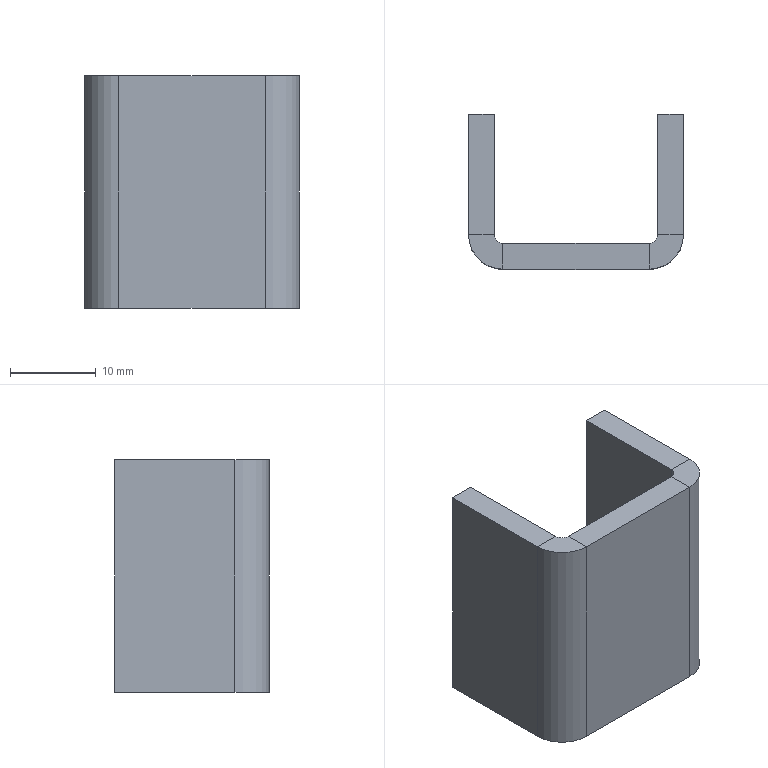Part | SolidWorks | features MirrorStock 1 | 1 solid | 22 faces | box 25 x 18 x 27 mm | volume 4281 mm3 | plane 18 | cylinder 4 | commonest cylinder face diameters 2 x2 8 x2
STEP:
#1=CARTESIAN_POINT('',(27.647,7.676,27.));
#2=VERTEX_POINT('',#1);
#3=CARTESIAN_POINT('',(27.647,10.676,27.));
#4=VERTEX_POINT('',#3);
#5=CARTESIAN_POINT('',(27.647,7.676,27.));
#6=DIRECTION('',(0.,1.,0.));
#7=VECTOR('',#6,1000.);
#8=LINE('',#5,#7);
#9=EDGE_CURVE('',#2,#4,#8,.T.);
#10=ORIENTED_EDGE('',*,*,#9,.T.);
#11=CARTESIAN_POINT('',(26.647,11.676,27.));
#12=VERTEX_POINT('',#11);
#13=CARTESIAN_POINT('',(27.647,11.676,27.));
#14=DIRECTION('',(0.,0.,1.));
#15=DIRECTION('',(1.,0.,0.));
#16=AXIS2_PLACEMENT_3D('',#13,#14,#15);
#17=CIRCLE('',#16,1.);
#18=EDGE_CURVE('',#12,#4,#17,.T.);
#19=ORIENTED_EDGE('',*,*,#18,.F.);
#20=CARTESIAN_POINT('',(23.647,11.676,27.));
#21=VERTEX_POINT('',#20);
#22=CARTESIAN_POINT('',(26.647,11.676,27.));
#23=DIRECTION('',(-1.,0.,0.));
#24=VECTOR('',#23,1000.);
#25=LINE('',#22,#24);
#26=EDGE_CURVE('',#12,#21,#25,.T.);
#27=ORIENTED_EDGE('',*,*,#26,.T.);
#28=CARTESIAN_POINT('',(27.647,11.676,27.));
#29=DIRECTION('',(0.,0.,1.));
#30=DIRECTION('',(-1.,0.,0.));
#31=AXIS2_PLACEMENT_3D('',#28,#29,#30);
#32=CIRCLE('',#31,4.);
#33=EDGE_CURVE('',#21,#2,#32,.T.);
#34=ORIENTED_EDGE('',*,*,#33,.T.);
#35=EDGE_LOOP('',(#10,#19,#27,#34));
#36=FACE_OUTER_BOUND('',#35,.T.);
#37=CARTESIAN_POINT('',(27.647,7.676,27.));
#38=DIRECTION('',(0.,0.,1.));
#39=DIRECTION('',(-1.,0.,0.));
#40=AXIS2_PLACEMENT_3D('',#37,#38,#39);
#41=PLANE('',#40);
#42=ADVANCED_FACE('',(#36),#41,.T.);
#43=CARTESIAN_POINT('',(44.647,7.676,27.));
#44=VERTEX_POINT('',#43);
#45=CARTESIAN_POINT('',(23.647,7.676,27.));
#46=DIRECTION('',(1.,0.,0.));
#47=VECTOR('',#46,1000.);
#48=LINE('',#45,#47);
#49=EDGE_CURVE('',#2,#44,#48,.T.);
#50=ORIENTED_EDGE('',*,*,#49,.T.);
#51=CARTESIAN_POINT('',(44.647,10.676,27.));
#52=VERTEX_POINT('',#51);
#53=CARTESIAN_POINT('',(44.647,10.676,27.));
#54=DIRECTION('',(0.,-1.,0.));
#55=VECTOR('',#54,1000.);
#56=LINE('',#53,#55);
#57=EDGE_CURVE('',#52,#44,#56,.T.);
#58=ORIENTED_EDGE('',*,*,#57,.F.);
#59=CARTESIAN_POINT('',(23.647,10.676,27.));
#60=DIRECTION('',(1.,0.,0.));
#61=VECTOR('',#60,1000.);
#62=LINE('',#59,#61);
#63=EDGE_CURVE('',#4,#52,#62,.T.);
#64=ORIENTED_EDGE('',*,*,#63,.F.);
#65=ORIENTED_EDGE('',*,*,#9,.F.);
#66=EDGE_LOOP('',(#50,#58,#64,#65));
#67=FACE_OUTER_BOUND('',#66,.T.);
#68=CARTESIAN_POINT('',(26.647,11.676,27.));
#69=DIRECTION('',(0.,0.,1.));
#70=DIRECTION('',(-1.,0.,0.));
#71=AXIS2_PLACEMENT_3D('',#68,#69,#70);
#72=PLANE('',#71);
#73=ADVANCED_FACE('',(#67),#72,.T.);
#74=CARTESIAN_POINT('',(23.647,11.676,0.));
#75=VERTEX_POINT('',#74);
#76=CARTESIAN_POINT('',(26.647,11.676,0.));
#77=VERTEX_POINT('',#76);
#78=CARTESIAN_POINT('',(23.647,11.676,0.));
#79=DIRECTION('',(1.,0.,0.));
#80=VECTOR('',#79,1000.);
#81=LINE('',#78,#80);
#82=EDGE_CURVE('',#75,#77,#81,.T.);
#83=ORIENTED_EDGE('',*,*,#82,.T.);
#84=CARTESIAN_POINT('',(27.647,10.676,0.));
#85=VERTEX_POINT('',#84);
#86=CARTESIAN_POINT('',(27.647,11.676,0.));
#87=DIRECTION('',(0.,0.,1.));
#88=DIRECTION('',(1.,0.,0.));
#89=AXIS2_PLACEMENT_3D('',#86,#87,#88);
#90=CIRCLE('',#89,1.);
#91=EDGE_CURVE('',#77,#85,#90,.T.);
#92=ORIENTED_EDGE('',*,*,#91,.T.);
#93=CARTESIAN_POINT('',(27.647,7.676,0.));
#94=VERTEX_POINT('',#93);
#95=CARTESIAN_POINT('',(27.647,10.676,0.));
#96=DIRECTION('',(0.,-1.,0.));
#97=VECTOR('',#96,1000.);
#98=LINE('',#95,#97);
#99=EDGE_CURVE('',#85,#94,#98,.T.);
#100=ORIENTED_EDGE('',*,*,#99,.T.);
#101=CARTESIAN_POINT('',(27.647,11.676,0.));
#102=DIRECTION('',(0.,0.,1.));
#103=DIRECTION('',(-1.,0.,0.));
#104=AXIS2_PLACEMENT_3D('',#101,#102,#103);
#105=CIRCLE('',#104,4.);
#106=EDGE_CURVE('',#75,#94,#105,.T.);
#107=ORIENTED_EDGE('',*,*,#106,.F.);
#108=EDGE_LOOP('',(#83,#92,#100,#107));
#109=FACE_OUTER_BOUND('',#108,.T.);
#110=CARTESIAN_POINT('',(23.647,11.676,0.));
#111=DIRECTION('',(0.,0.,-1.));
#112=DIRECTION('',(1.,0.,0.));
#113=AXIS2_PLACEMENT_3D('',#110,#111,#112);
#114=PLANE('',#113);
#115=ADVANCED_FACE('',(#109),#114,.T.);
#116=CARTESIAN_POINT('',(23.647,25.676,0.));
#117=VERTEX_POINT('',#116);
#118=CARTESIAN_POINT('',(23.647,25.676,0.));
#119=DIRECTION('',(0.,-1.,0.));
#120=VECTOR('',#119,1000.);
#121=LINE('',#118,#120);
#122=EDGE_CURVE('',#117,#75,#121,.T.);
#123=ORIENTED_EDGE('',*,*,#122,.F.);
#124=CARTESIAN_POINT('',(26.647,25.676,0.));
#125=VERTEX_POINT('',#124);
#126=CARTESIAN_POINT('',(23.647,25.676,0.));
#127=DIRECTION('',(1.,0.,0.));
#128=VECTOR('',#127,1000.);
#129=LINE('',#126,#128);
#130=EDGE_CURVE('',#117,#125,#129,.T.);
#131=ORIENTED_EDGE('',*,*,#130,.T.);
#132=CARTESIAN_POINT('',(26.647,25.676,0.));
#133=DIRECTION('',(0.,-1.,0.));
#134=VECTOR('',#133,1000.);
#135=LINE('',#132,#134);
#136=EDGE_CURVE('',#125,#77,#135,.T.);
#137=ORIENTED_EDGE('',*,*,#136,.T.);
#138=ORIENTED_EDGE('',*,*,#82,.F.);
#139=EDGE_LOOP('',(#123,#131,#137,#138));
#140=FACE_OUTER_BOUND('',#139,.T.);
#141=CARTESIAN_POINT('',(27.647,10.676,0.));
#142=DIRECTION('',(0.,0.,-1.));
#143=DIRECTION('',(1.,0.,0.));
#144=AXIS2_PLACEMENT_3D('',#141,#142,#143);
#145=PLANE('',#144);
#146=ADVANCED_FACE('',(#140),#145,.T.);
#147=CARTESIAN_POINT('',(48.647,11.676,27.));
#148=VERTEX_POINT('',#147);
#149=CARTESIAN_POINT('',(45.647,11.676,27.));
#150=VERTEX_POINT('',#149);
#151=CARTESIAN_POINT('',(48.647,11.676,27.));
#152=DIRECTION('',(-1.,0.,0.));
#153=VECTOR('',#152,1000.);
#154=LINE('',#151,#153);
#155=EDGE_CURVE('',#148,#150,#154,.T.);
#156=ORIENTED_EDGE('',*,*,#155,.T.);
#157=CARTESIAN_POINT('',(44.647,11.676,27.));
#158=DIRECTION('',(0.,0.,1.));
#159=DIRECTION('',(1.,0.,0.));
#160=AXIS2_PLACEMENT_3D('',#157,#158,#159);
#161=CIRCLE('',#160,1.);
#162=EDGE_CURVE('',#52,#150,#161,.T.);
#163=ORIENTED_EDGE('',*,*,#162,.F.);
#164=ORIENTED_EDGE('',*,*,#57,.T.);
#165=CARTESIAN_POINT('',(44.647,11.676,27.));
#166=DIRECTION('',(0.,0.,1.));
#167=DIRECTION('',(-1.,0.,0.));
#168=AXIS2_PLACEMENT_3D('',#165,#166,#167);
#169=CIRCLE('',#168,4.);
#170=EDGE_CURVE('',#44,#148,#169,.T.);
#171=ORIENTED_EDGE('',*,*,#170,.T.);
#172=EDGE_LOOP('',(#156,#163,#164,#171));
#173=FACE_OUTER_BOUND('',#172,.T.);
#174=CARTESIAN_POINT('',(48.647,11.676,27.));
#175=DIRECTION('',(0.,0.,1.));
#176=DIRECTION('',(-1.,0.,0.));
#177=AXIS2_PLACEMENT_3D('',#174,#175,#176);
#178=PLANE('',#177);
#179=ADVANCED_FACE('',(#173),#178,.T.);
#180=CARTESIAN_POINT('',(48.647,25.676,27.));
#181=VERTEX_POINT('',#180);
#182=CARTESIAN_POINT('',(48.647,7.676,27.));
#183=DIRECTION('',(0.,1.,0.));
#184=VECTOR('',#183,1000.);
#185=LINE('',#182,#184);
#186=EDGE_CURVE('',#148,#181,#185,.T.);
#187=ORIENTED_EDGE('',*,*,#186,.T.);
#188=CARTESIAN_POINT('',(45.647,25.676,27.));
#189=VERTEX_POINT('',#188);
#190=CARTESIAN_POINT('',(45.647,25.676,27.));
#191=DIRECTION('',(1.,0.,0.));
#192=VECTOR('',#191,1000.);
#193=LINE('',#190,#192);
#194=EDGE_CURVE('',#189,#181,#193,.T.);
#195=ORIENTED_EDGE('',*,*,#194,.F.);
#196=CARTESIAN_POINT('',(45.647,7.676,27.));
#197=DIRECTION('',(0.,1.,0.));
#198=VECTOR('',#197,1000.);
#199=LINE('',#196,#198);
#200=EDGE_CURVE('',#150,#189,#199,.T.);
#201=ORIENTED_EDGE('',*,*,#200,.F.);
#202=ORIENTED_EDGE('',*,*,#155,.F.);
#203=EDGE_LOOP('',(#187,#195,#201,#202));
#204=FACE_OUTER_BOUND('',#203,.T.);
#205=CARTESIAN_POINT('',(44.647,10.676,27.));
#206=DIRECTION('',(0.,0.,1.));
#207=DIRECTION('',(-1.,0.,0.));
#208=AXIS2_PLACEMENT_3D('',#205,#206,#207);
#209=PLANE('',#208);
#210=ADVANCED_FACE('',(#204),#209,.T.);
#211=CARTESIAN_POINT('',(44.647,7.676,0.));
#212=VERTEX_POINT('',#211);
#213=CARTESIAN_POINT('',(44.647,10.676,0.));
#214=VERTEX_POINT('',#213);
#215=CARTESIAN_POINT('',(44.647,7.676,0.));
#216=DIRECTION('',(0.,1.,0.));
#217=VECTOR('',#216,1000.);
#218=LINE('',#215,#217);
#219=EDGE_CURVE('',#212,#214,#218,.T.);
#220=ORIENTED_EDGE('',*,*,#219,.T.);
#221=CARTESIAN_POINT('',(45.647,11.676,0.));
#222=VERTEX_POINT('',#221);
#223=CARTESIAN_POINT('',(44.647,11.676,0.));
#224=DIRECTION('',(0.,0.,1.));
#225=DIRECTION('',(1.,0.,0.));
#226=AXIS2_PLACEMENT_3D('',#223,#224,#225);
#227=CIRCLE('',#226,1.);
#228=EDGE_CURVE('',#214,#222,#227,.T.);
#229=ORIENTED_EDGE('',*,*,#228,.T.);
#230=CARTESIAN_POINT('',(48.647,11.676,0.));
#231=VERTEX_POINT('',#230);
#232=CARTESIAN_POINT('',(45.647,11.676,0.));
#233=DIRECTION('',(1.,0.,0.));
#234=VECTOR('',#233,1000.);
#235=LINE('',#232,#234);
#236=EDGE_CURVE('',#222,#231,#235,.T.);
#237=ORIENTED_EDGE('',*,*,#236,.T.);
#238=CARTESIAN_POINT('',(44.647,11.676,0.));
#239=DIRECTION('',(0.,0.,1.));
#240=DIRECTION('',(-1.,0.,0.));
#241=AXIS2_PLACEMENT_3D('',#238,#239,#240);
#242=CIRCLE('',#241,4.);
#243=EDGE_CURVE('',#212,#231,#242,.T.);
#244=ORIENTED_EDGE('',*,*,#243,.F.);
#245=EDGE_LOOP('',(#220,#229,#237,#244));
#246=FACE_OUTER_BOUND('',#245,.T.);
#247=CARTESIAN_POINT('',(44.647,7.676,0.));
#248=DIRECTION('',(0.,0.,-1.));
#249=DIRECTION('',(1.,0.,0.));
#250=AXIS2_PLACEMENT_3D('',#247,#248,#249);
#251=PLANE('',#250);
#252=ADVANCED_FACE('',(#246),#251,.T.);
#253=CARTESIAN_POINT('',(23.647,7.676,0.));
#254=DIRECTION('',(1.,0.,0.));
#255=VECTOR('',#254,1000.);
#256=LINE('',#253,#255);
#257=EDGE_CURVE('',#94,#212,#256,.T.);
#258=ORIENTED_EDGE('',*,*,#257,.F.);
#259=ORIENTED_EDGE('',*,*,#99,.F.);
#260=CARTESIAN_POINT('',(23.647,10.676,0.));
#261=DIRECTION('',(1.,0.,0.));
#262=VECTOR('',#261,1000.);
#263=LINE('',#260,#262);
#264=EDGE_CURVE('',#85,#214,#263,.T.);
#265=ORIENTED_EDGE('',*,*,#264,.T.);
#266=ORIENTED_EDGE('',*,*,#219,.F.);
#267=EDGE_LOOP('',(#258,#259,#265,#266));
#268=FACE_OUTER_BOUND('',#267,.T.);
#269=CARTESIAN_POINT('',(45.647,11.676,0.));
#270=DIRECTION('',(0.,0.,-1.));
#271=DIRECTION('',(1.,0.,0.));
#272=AXIS2_PLACEMENT_3D('',#269,#270,#271);
#273=PLANE('',#272);
#274=ADVANCED_FACE('',(#268),#273,.T.);
#275=CARTESIAN_POINT('',(48.647,25.676,0.));
#276=VERTEX_POINT('',#275);
#277=CARTESIAN_POINT('',(48.647,7.676,0.));
#278=DIRECTION('',(0.,1.,0.));
#279=VECTOR('',#278,1000.);
#280=LINE('',#277,#279);
#281=EDGE_CURVE('',#231,#276,#280,.T.);
#282=ORIENTED_EDGE('',*,*,#281,.T.);
#283=CARTESIAN_POINT('',(48.647,25.676,27.));
#284=DIRECTION('',(0.,0.,-1.));
#285=VECTOR('',#284,1000.);
#286=LINE('',#283,#285);
#287=EDGE_CURVE('',#181,#276,#286,.T.);
#288=ORIENTED_EDGE('',*,*,#287,.F.);
#289=ORIENTED_EDGE('',*,*,#186,.F.);
#290=CARTESIAN_POINT('',(48.647,11.676,27.));
#291=DIRECTION('',(0.,0.,-1.));
#292=VECTOR('',#291,1000.);
#293=LINE('',#290,#292);
#294=EDGE_CURVE('',#148,#231,#293,.T.);
#295=ORIENTED_EDGE('',*,*,#294,.T.);
#296=EDGE_LOOP('',(#282,#288,#289,#295));
#297=FACE_OUTER_BOUND('',#296,.T.);
#298=CARTESIAN_POINT('',(48.647,7.676,27.));
#299=DIRECTION('',(1.,0.,0.));
#300=DIRECTION('',(0.,0.,1.));
#301=AXIS2_PLACEMENT_3D('',#298,#299,#300);
#302=PLANE('',#301);
#303=ADVANCED_FACE('',(#297),#302,.T.);
#304=ORIENTED_EDGE('',*,*,#243,.T.);
#305=ORIENTED_EDGE('',*,*,#294,.F.);
#306=ORIENTED_EDGE('',*,*,#170,.F.);
#307=CARTESIAN_POINT('',(44.647,7.676,27.));
#308=DIRECTION('',(0.,0.,-1.));
#309=VECTOR('',#308,1000.);
#310=LINE('',#307,#309);
#311=EDGE_CURVE('',#44,#212,#310,.T.);
#312=ORIENTED_EDGE('',*,*,#311,.T.);
#313=EDGE_LOOP('',(#304,#305,#306,#312));
#314=FACE_OUTER_BOUND('',#313,.T.);
#315=CARTESIAN_POINT('',(44.647,11.676,27.));
#316=DIRECTION('',(0.,0.,-1.));
#317=DIRECTION('',(1.,0.,0.));
#318=AXIS2_PLACEMENT_3D('',#315,#316,#317);
#319=CYLINDRICAL_SURFACE('',#318,4.);
#320=ADVANCED_FACE('',(#314),#319,.T.);
#321=ORIENTED_EDGE('',*,*,#257,.T.);
#322=ORIENTED_EDGE('',*,*,#311,.F.);
#323=ORIENTED_EDGE('',*,*,#49,.F.);
#324=CARTESIAN_POINT('',(27.647,7.676,27.));
#325=DIRECTION('',(0.,0.,-1.));
#326=VECTOR('',#325,1000.);
#327=LINE('',#324,#326);
#328=EDGE_CURVE('',#2,#94,#327,.T.);
#329=ORIENTED_EDGE('',*,*,#328,.T.);
#330=EDGE_LOOP('',(#321,#322,#323,#329));
#331=FACE_OUTER_BOUND('',#330,.T.);
#332=CARTESIAN_POINT('',(23.647,7.676,27.));
#333=DIRECTION('',(0.,-1.,0.));
#334=DIRECTION('',(0.,0.,1.));
#335=AXIS2_PLACEMENT_3D('',#332,#333,#334);
#336=PLANE('',#335);
#337=ADVANCED_FACE('',(#331),#336,.T.);
#338=ORIENTED_EDGE('',*,*,#106,.T.);
#339=ORIENTED_EDGE('',*,*,#328,.F.);
#340=ORIENTED_EDGE('',*,*,#33,.F.);
#341=CARTESIAN_POINT('',(23.647,11.676,27.));
#342=DIRECTION('',(0.,0.,-1.));
#343=VECTOR('',#342,1000.);
#344=LINE('',#341,#343);
#345=EDGE_CURVE('',#21,#75,#344,.T.);
#346=ORIENTED_EDGE('',*,*,#345,.T.);
#347=EDGE_LOOP('',(#338,#339,#340,#346));
#348=FACE_OUTER_BOUND('',#347,.T.);
#349=CARTESIAN_POINT('',(27.647,11.676,27.));
#350=DIRECTION('',(0.,0.,-1.));
#351=DIRECTION('',(1.,0.,0.));
#352=AXIS2_PLACEMENT_3D('',#349,#350,#351);
#353=CYLINDRICAL_SURFACE('',#352,4.);
#354=ADVANCED_FACE('',(#348),#353,.T.);
#355=ORIENTED_EDGE('',*,*,#122,.T.);
#356=ORIENTED_EDGE('',*,*,#345,.F.);
#357=CARTESIAN_POINT('',(23.647,25.676,27.));
#358=VERTEX_POINT('',#357);
#359=CARTESIAN_POINT('',(23.647,25.676,27.));
#360=DIRECTION('',(0.,-1.,0.));
#361=VECTOR('',#360,1000.);
#362=LINE('',#359,#361);
#363=EDGE_CURVE('',#358,#21,#362,.T.);
#364=ORIENTED_EDGE('',*,*,#363,.F.);
#365=CARTESIAN_POINT('',(23.647,25.676,27.));
#366=DIRECTION('',(0.,0.,-1.));
#367=VECTOR('',#366,1000.);
#368=LINE('',#365,#367);
#369=EDGE_CURVE('',#358,#117,#368,.T.);
#370=ORIENTED_EDGE('',*,*,#369,.T.);
#371=EDGE_LOOP('',(#355,#356,#364,#370));
#372=FACE_OUTER_BOUND('',#371,.T.);
#373=CARTESIAN_POINT('',(23.647,25.676,27.));
#374=DIRECTION('',(-1.,0.,0.));
#375=DIRECTION('',(0.,0.,-1.));
#376=AXIS2_PLACEMENT_3D('',#373,#374,#375);
#377=PLANE('',#376);
#378=ADVANCED_FACE('',(#372),#377,.T.);
#379=ORIENTED_EDGE('',*,*,#130,.F.);
#380=ORIENTED_EDGE('',*,*,#369,.F.);
#381=CARTESIAN_POINT('',(26.647,25.676,27.));
#382=VERTEX_POINT('',#381);
#383=CARTESIAN_POINT('',(23.647,25.676,27.));
#384=DIRECTION('',(1.,0.,0.));
#385=VECTOR('',#384,1000.);
#386=LINE('',#383,#385);
#387=EDGE_CURVE('',#358,#382,#386,.T.);
#388=ORIENTED_EDGE('',*,*,#387,.T.);
#389=CARTESIAN_POINT('',(26.647,25.676,27.));
#390=DIRECTION('',(0.,0.,-1.));
#391=VECTOR('',#390,1000.);
#392=LINE('',#389,#391);
#393=EDGE_CURVE('',#382,#125,#392,.T.);
#394=ORIENTED_EDGE('',*,*,#393,.T.);
#395=EDGE_LOOP('',(#379,#380,#388,#394));
#396=FACE_OUTER_BOUND('',#395,.T.);
#397=CARTESIAN_POINT('',(23.647,25.676,27.));
#398=DIRECTION('',(0.,-1.,0.));
#399=DIRECTION('',(0.,0.,1.));
#400=AXIS2_PLACEMENT_3D('',#397,#398,#399);
#401=PLANE('',#400);
#402=ADVANCED_FACE('',(#396),#401,.F.);
#403=ORIENTED_EDGE('',*,*,#136,.F.);
#404=ORIENTED_EDGE('',*,*,#393,.F.);
#405=CARTESIAN_POINT('',(26.647,25.676,27.));
#406=DIRECTION('',(0.,-1.,0.));
#407=VECTOR('',#406,1000.);
#408=LINE('',#405,#407);
#409=EDGE_CURVE('',#382,#12,#408,.T.);
#410=ORIENTED_EDGE('',*,*,#409,.T.);
#411=CARTESIAN_POINT('',(26.647,11.676,27.));
#412=DIRECTION('',(0.,0.,-1.));
#413=VECTOR('',#412,1000.);
#414=LINE('',#411,#413);
#415=EDGE_CURVE('',#12,#77,#414,.T.);
#416=ORIENTED_EDGE('',*,*,#415,.T.);
#417=EDGE_LOOP('',(#403,#404,#410,#416));
#418=FACE_OUTER_BOUND('',#417,.T.);
#419=CARTESIAN_POINT('',(26.647,25.676,27.));
#420=DIRECTION('',(-1.,0.,0.));
#421=DIRECTION('',(0.,0.,-1.));
#422=AXIS2_PLACEMENT_3D('',#419,#420,#421);
#423=PLANE('',#422);
#424=ADVANCED_FACE('',(#418),#423,.F.);
#425=ORIENTED_EDGE('',*,*,#91,.F.);
#426=ORIENTED_EDGE('',*,*,#415,.F.);
#427=ORIENTED_EDGE('',*,*,#18,.T.);
#428=CARTESIAN_POINT('',(27.647,10.676,27.));
#429=DIRECTION('',(0.,0.,-1.));
#430=VECTOR('',#429,1000.);
#431=LINE('',#428,#430);
#432=EDGE_CURVE('',#4,#85,#431,.T.);
#433=ORIENTED_EDGE('',*,*,#432,.T.);
#434=EDGE_LOOP('',(#425,#426,#427,#433));
#435=FACE_OUTER_BOUND('',#434,.T.);
#436=CARTESIAN_POINT('',(27.647,11.676,27.));
#437=DIRECTION('',(0.,0.,-1.));
#438=DIRECTION('',(1.,0.,0.));
#439=AXIS2_PLACEMENT_3D('',#436,#437,#438);
#440=CYLINDRICAL_SURFACE('',#439,1.);
#441=ADVANCED_FACE('',(#435),#440,.F.);
#442=ORIENTED_EDGE('',*,*,#264,.F.);
#443=ORIENTED_EDGE('',*,*,#432,.F.);
#444=ORIENTED_EDGE('',*,*,#63,.T.);
#445=CARTESIAN_POINT('',(44.647,10.676,27.));
#446=DIRECTION('',(0.,0.,-1.));
#447=VECTOR('',#446,1000.);
#448=LINE('',#445,#447);
#449=EDGE_CURVE('',#52,#214,#448,.T.);
#450=ORIENTED_EDGE('',*,*,#449,.T.);
#451=EDGE_LOOP('',(#442,#443,#444,#450));
#452=FACE_OUTER_BOUND('',#451,.T.);
#453=CARTESIAN_POINT('',(23.647,10.676,27.));
#454=DIRECTION('',(0.,-1.,0.));
#455=DIRECTION('',(0.,0.,1.));
#456=AXIS2_PLACEMENT_3D('',#453,#454,#455);
#457=PLANE('',#456);
#458=ADVANCED_FACE('',(#452),#457,.F.);
#459=ORIENTED_EDGE('',*,*,#228,.F.);
#460=ORIENTED_EDGE('',*,*,#449,.F.);
#461=ORIENTED_EDGE('',*,*,#162,.T.);
#462=CARTESIAN_POINT('',(45.647,11.676,27.));
#463=DIRECTION('',(0.,0.,-1.));
#464=VECTOR('',#463,1000.);
#465=LINE('',#462,#464);
#466=EDGE_CURVE('',#150,#222,#465,.T.);
#467=ORIENTED_EDGE('',*,*,#466,.T.);
#468=EDGE_LOOP('',(#459,#460,#461,#467));
#469=FACE_OUTER_BOUND('',#468,.T.);
#470=CARTESIAN_POINT('',(44.647,11.676,27.));
#471=DIRECTION('',(0.,0.,-1.));
#472=DIRECTION('',(1.,0.,0.));
#473=AXIS2_PLACEMENT_3D('',#470,#471,#472);
#474=CYLINDRICAL_SURFACE('',#473,1.);
#475=ADVANCED_FACE('',(#469),#474,.F.);
#476=CARTESIAN_POINT('',(45.647,25.676,0.));
#477=VERTEX_POINT('',#476);
#478=CARTESIAN_POINT('',(45.647,7.676,0.));
#479=DIRECTION('',(0.,1.,0.));
#480=VECTOR('',#479,1000.);
#481=LINE('',#478,#480);
#482=EDGE_CURVE('',#222,#477,#481,.T.);
#483=ORIENTED_EDGE('',*,*,#482,.F.);
#484=ORIENTED_EDGE('',*,*,#466,.F.);
#485=ORIENTED_EDGE('',*,*,#200,.T.);
#486=CARTESIAN_POINT('',(45.647,25.676,27.));
#487=DIRECTION('',(0.,0.,-1.));
#488=VECTOR('',#487,1000.);
#489=LINE('',#486,#488);
#490=EDGE_CURVE('',#189,#477,#489,.T.);
#491=ORIENTED_EDGE('',*,*,#490,.T.);
#492=EDGE_LOOP('',(#483,#484,#485,#491));
#493=FACE_OUTER_BOUND('',#492,.T.);
#494=CARTESIAN_POINT('',(45.647,7.676,27.));
#495=DIRECTION('',(1.,0.,0.));
#496=DIRECTION('',(0.,0.,1.));
#497=AXIS2_PLACEMENT_3D('',#494,#495,#496);
#498=PLANE('',#497);
#499=ADVANCED_FACE('',(#493),#498,.F.);
#500=CARTESIAN_POINT('',(45.647,25.676,0.));
#501=DIRECTION('',(1.,0.,0.));
#502=VECTOR('',#501,1000.);
#503=LINE('',#500,#502);
#504=EDGE_CURVE('',#477,#276,#503,.T.);
#505=ORIENTED_EDGE('',*,*,#504,.F.);
#506=ORIENTED_EDGE('',*,*,#490,.F.);
#507=ORIENTED_EDGE('',*,*,#194,.T.);
#508=ORIENTED_EDGE('',*,*,#287,.T.);
#509=EDGE_LOOP('',(#505,#506,#507,#508));
#510=FACE_OUTER_BOUND('',#509,.T.);
#511=CARTESIAN_POINT('',(45.647,25.676,27.));
#512=DIRECTION('',(0.,-1.,0.));
#513=DIRECTION('',(0.,0.,1.));
#514=AXIS2_PLACEMENT_3D('',#511,#512,#513);
#515=PLANE('',#514);
#516=ADVANCED_FACE('',(#510),#515,.F.);
#517=ORIENTED_EDGE('',*,*,#409,.F.);
#518=ORIENTED_EDGE('',*,*,#387,.F.);
#519=ORIENTED_EDGE('',*,*,#363,.T.);
#520=ORIENTED_EDGE('',*,*,#26,.F.);
#521=EDGE_LOOP('',(#517,#518,#519,#520));
#522=FACE_OUTER_BOUND('',#521,.T.);
#523=CARTESIAN_POINT('',(44.647,11.676,27.));
#524=DIRECTION('',(0.,0.,-1.));
#525=DIRECTION('',(1.,0.,0.));
#526=AXIS2_PLACEMENT_3D('',#523,#524,#525);
#527=PLANE('',#526);
#528=ADVANCED_FACE('',(#522),#527,.F.);
#529=ORIENTED_EDGE('',*,*,#281,.F.);
#530=ORIENTED_EDGE('',*,*,#236,.F.);
#531=ORIENTED_EDGE('',*,*,#482,.T.);
#532=ORIENTED_EDGE('',*,*,#504,.T.);
#533=EDGE_LOOP('',(#529,#530,#531,#532));
#534=FACE_OUTER_BOUND('',#533,.T.);
#535=CARTESIAN_POINT('',(44.647,11.676,0.));
#536=DIRECTION('',(0.,0.,-1.));
#537=DIRECTION('',(1.,0.,0.));
#538=AXIS2_PLACEMENT_3D('',#535,#536,#537);
#539=PLANE('',#538);
#540=ADVANCED_FACE('',(#534),#539,.T.);
#541=CLOSED_SHELL('',(#42,#73,#115,#146,#179,#210,#252,#274,#303,#320,#337,#354,#378,#402,#424,#441,#458,#475,#499,#516,#528,#540));
#542=MANIFOLD_SOLID_BREP('',#541);
#543=CARTESIAN_POINT('',(0.,0.,0.));
#544=DIRECTION('',(0.,0.,1.));
#545=DIRECTION('',(1.,0.,0.));
#546=AXIS2_PLACEMENT_3D('',#543,#544,#545);
#547=(LENGTH_UNIT()NAMED_UNIT(*)SI_UNIT(.MILLI.,.METRE.));
#548=UNCERTAINTY_MEASURE_WITH_UNIT(LENGTH_MEASURE(0.00001),#547,'','');
#549=(NAMED_UNIT(*)PLANE_ANGLE_UNIT()SI_UNIT($,.RADIAN.));
#550=(NAMED_UNIT(*)SI_UNIT($,.STERADIAN.)SOLID_ANGLE_UNIT());
#551=(GEOMETRIC_REPRESENTATION_CONTEXT(3)GLOBAL_UNCERTAINTY_ASSIGNED_CONTEXT((#548))GLOBAL_UNIT_ASSIGNED_CONTEXT((#547,#549,#550))REPRESENTATION_CONTEXT('',''));
#552=ADVANCED_BREP_SHAPE_REPRESENTATION('',(#542,#546),#551);